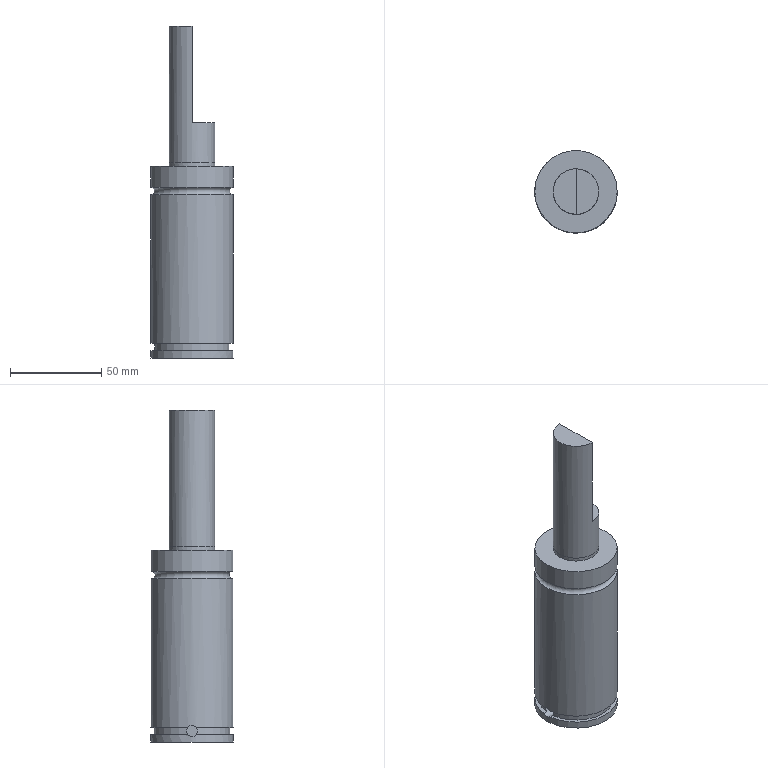Part | NX | features solid 2 | 1 solid | 16 faces | box 45.2 x 45.2 x 182 mm | volume 191111 mm3 | plane 8 | cylinder 7 | torus 1 | commonest cylinder face diameters 45.2 x3 6 x1 24.98 x1 25 x1 41.2 x1
STEP:
#1=CARTESIAN_POINT('',(-447.489,-357.236,-202.));
#2=VERTEX_POINT('',#1);
#3=CARTESIAN_POINT('',(-447.489,-352.764,-202.));
#4=VERTEX_POINT('',#3);
#5=CARTESIAN_POINT('',(-425.,-355.,-202.));
#6=DIRECTION('',(0.,0.,-1.));
#7=DIRECTION('',(1.,0.,0.));
#8=AXIS2_PLACEMENT_3D('',#5,#6,#7);
#9=CIRCLE('',#8,22.6);
#10=EDGE_CURVE('',#2,#4,#9,.F.);
#11=ORIENTED_EDGE('',*,*,#10,.T.);
#12=CARTESIAN_POINT('',(-447.489,-352.764,-202.));
#13=CARTESIAN_POINT('',(-447.545,-353.325,-201.372));
#14=CARTESIAN_POINT('',(-447.655,-355.003,-200.628));
#15=CARTESIAN_POINT('',(-447.545,-356.675,-201.372));
#16=CARTESIAN_POINT('',(-447.489,-357.236,-202.));
#17=B_SPLINE_CURVE_WITH_KNOTS('',3,(#12,#13,#14,#15,#16),.UNSPECIFIED.,.F.,.F.,(4,1,4),(0.006877,0.009391,0.01191),.UNSPECIFIED.);
#18=EDGE_CURVE('',#4,#2,#17,.T.);
#19=ORIENTED_EDGE('',*,*,#18,.T.);
#20=EDGE_LOOP('',(#11,#19));
#21=FACE_BOUND('',#20,.T.);
#22=CARTESIAN_POINT('',(-402.4,-355.,-120.5));
#23=VERTEX_POINT('',#22);
#24=CARTESIAN_POINT('',(-425.,-355.,-120.5));
#25=DIRECTION('',(0.,0.,-1.));
#26=DIRECTION('',(1.,0.,0.));
#27=AXIS2_PLACEMENT_3D('',#24,#25,#26);
#28=CIRCLE('',#27,22.6);
#29=EDGE_CURVE('',#23,#23,#28,.T.);
#30=ORIENTED_EDGE('',*,*,#29,.T.);
#31=EDGE_LOOP('',(#30));
#32=FACE_BOUND('',#31,.T.);
#33=CARTESIAN_POINT('',(-425.,-355.,-105.));
#34=DIRECTION('',(0.,0.,-1.));
#35=DIRECTION('',(1.,0.,0.));
#36=AXIS2_PLACEMENT_3D('',#33,#34,#35);
#37=CYLINDRICAL_SURFACE('',#36,22.6);
#38=ADVANCED_FACE('',(#21,#32),#37,.T.);
#39=CARTESIAN_POINT('',(-447.6,-355.,-105.));
#40=VERTEX_POINT('',#39);
#41=CARTESIAN_POINT('',(-425.,-355.,-105.));
#42=DIRECTION('',(0.,0.,1.));
#43=DIRECTION('',(-1.,0.,0.));
#44=AXIS2_PLACEMENT_3D('',#41,#42,#43);
#45=CIRCLE('',#44,22.6);
#46=EDGE_CURVE('',#40,#40,#45,.T.);
#47=ORIENTED_EDGE('',*,*,#46,.T.);
#48=EDGE_LOOP('',(#47));
#49=FACE_BOUND('',#48,.T.);
#50=CARTESIAN_POINT('',(-437.5,-355.,-105.));
#51=VERTEX_POINT('',#50);
#52=CARTESIAN_POINT('',(-425.,-355.,-105.));
#53=DIRECTION('',(0.,0.,1.));
#54=DIRECTION('',(-1.,0.,0.));
#55=AXIS2_PLACEMENT_3D('',#52,#53,#54);
#56=CIRCLE('',#55,12.5);
#57=EDGE_CURVE('',#51,#51,#56,.T.);
#58=ORIENTED_EDGE('',*,*,#57,.F.);
#59=EDGE_LOOP('',(#58));
#60=FACE_BOUND('',#59,.T.);
#61=CARTESIAN_POINT('',(-425.,-355.,-105.));
#62=DIRECTION('',(0.,0.,1.));
#63=DIRECTION('',(-1.,0.,0.));
#64=AXIS2_PLACEMENT_3D('',#61,#62,#63);
#65=PLANE('',#64);
#66=ADVANCED_FACE('',(#49,#60),#65,.T.);
#67=CARTESIAN_POINT('',(-402.4,-355.,-116.5));
#68=VERTEX_POINT('',#67);
#69=CARTESIAN_POINT('',(-425.,-355.,-116.5));
#70=DIRECTION('',(0.,0.,-1.));
#71=DIRECTION('',(1.,0.,0.));
#72=AXIS2_PLACEMENT_3D('',#69,#70,#71);
#73=CIRCLE('',#72,22.6);
#74=EDGE_CURVE('',#68,#68,#73,.F.);
#75=ORIENTED_EDGE('',*,*,#74,.T.);
#76=EDGE_LOOP('',(#75));
#77=FACE_BOUND('',#76,.T.);
#78=ORIENTED_EDGE('',*,*,#46,.F.);
#79=EDGE_LOOP('',(#78));
#80=FACE_BOUND('',#79,.T.);
#81=CARTESIAN_POINT('',(-425.,-355.,-105.));
#82=DIRECTION('',(0.,0.,-1.));
#83=DIRECTION('',(1.,0.,0.));
#84=AXIS2_PLACEMENT_3D('',#81,#82,#83);
#85=CYLINDRICAL_SURFACE('',#84,22.6);
#86=ADVANCED_FACE('',(#77,#80),#85,.T.);
#87=CARTESIAN_POINT('',(-433.818,-346.154,-103.));
#88=VERTEX_POINT('',#87);
#89=CARTESIAN_POINT('',(-438.852,-354.978,-103.));
#90=CARTESIAN_POINT('',(-434.78,-345.19,-103.));
#91=CARTESIAN_POINT('',(-424.978,-341.148,-103.));
#92=CARTESIAN_POINT('',(-415.19,-345.22,-103.));
#93=CARTESIAN_POINT('',(-411.148,-355.022,-103.));
#94=CARTESIAN_POINT('',(-415.22,-364.81,-103.));
#95=CARTESIAN_POINT('',(-425.022,-368.852,-103.));
#96=CARTESIAN_POINT('',(-434.81,-364.78,-103.));
#97=CARTESIAN_POINT('',(-438.852,-354.978,-103.));
#98=CARTESIAN_POINT('',(-434.78,-345.19,-103.));
#99=CARTESIAN_POINT('',(-424.978,-341.148,-103.));
#100=B_SPLINE_CURVE_WITH_KNOTS('',3,(#89,#90,#91,#92,#93,#94,#95,#96,#97,#98,#99),.UNSPECIFIED.,.T.,.F.,(1,1,1,1,1,1,1,1,1,1,1,1,1,1,1),(-0.2498,-0.1248,0.0002479,0.1252,0.2502,0.3752,0.5002,0.6252,0.7502,0.8752,1.,1.125,1.25,1.375,1.5),.UNSPECIFIED.);
#101=EDGE_CURVE('',#88,#88,#100,.F.);
#102=ORIENTED_EDGE('',*,*,#101,.F.);
#103=EDGE_LOOP('',(#102));
#104=FACE_BOUND('',#103,.T.);
#105=ORIENTED_EDGE('',*,*,#57,.T.);
#106=EDGE_LOOP('',(#105));
#107=FACE_BOUND('',#106,.T.);
#108=CARTESIAN_POINT('',(-425.,-355.,-103.));
#109=DIRECTION('',(0.,0.,-1.));
#110=DIRECTION('',(1.,0.,0.));
#111=AXIS2_PLACEMENT_3D('',#108,#109,#110);
#112=CYLINDRICAL_SURFACE('',#111,12.5);
#113=ADVANCED_FACE('',(#104,#107),#112,.T.);
#114=ORIENTED_EDGE('',*,*,#74,.F.);
#115=EDGE_LOOP('',(#114));
#116=FACE_BOUND('',#115,.T.);
#117=ORIENTED_EDGE('',*,*,#29,.F.);
#118=EDGE_LOOP('',(#117));
#119=FACE_BOUND('',#118,.T.);
#120=CARTESIAN_POINT('',(-425.,-355.,-118.5));
#121=DIRECTION('',(0.,0.,-1.));
#122=DIRECTION('',(1.,0.,0.));
#123=AXIS2_PLACEMENT_3D('',#120,#121,#122);
#124=TOROIDAL_SURFACE('',#123,22.6,2.);
#125=ADVANCED_FACE('',(#116,#119),#124,.F.);
#126=ORIENTED_EDGE('',*,*,#10,.F.);
#127=CARTESIAN_POINT('',(-445.478,-357.236,-202.));
#128=VERTEX_POINT('',#127);
#129=CARTESIAN_POINT('',(-440.1,-357.236,-202.));
#130=DIRECTION('',(-1.,0.,0.));
#131=VECTOR('',#130,1000.);
#132=LINE('',#129,#131);
#133=EDGE_CURVE('',#2,#128,#132,.F.);
#134=ORIENTED_EDGE('',*,*,#133,.T.);
#135=CARTESIAN_POINT('',(-445.478,-352.764,-202.));
#136=VERTEX_POINT('',#135);
#137=CARTESIAN_POINT('',(-425.,-355.,-202.));
#138=DIRECTION('',(0.,0.,1.));
#139=DIRECTION('',(-1.,0.,0.));
#140=AXIS2_PLACEMENT_3D('',#137,#138,#139);
#141=CIRCLE('',#140,20.6);
#142=EDGE_CURVE('',#128,#136,#141,.T.);
#143=ORIENTED_EDGE('',*,*,#142,.T.);
#144=CARTESIAN_POINT('',(-440.1,-352.764,-202.));
#145=DIRECTION('',(-1.,0.,0.));
#146=VECTOR('',#145,1000.);
#147=LINE('',#144,#146);
#148=EDGE_CURVE('',#136,#4,#147,.T.);
#149=ORIENTED_EDGE('',*,*,#148,.T.);
#150=EDGE_LOOP('',(#126,#134,#143,#149));
#151=FACE_BOUND('',#150,.T.);
#152=CARTESIAN_POINT('',(-425.,-355.,-202.));
#153=DIRECTION('',(0.,0.,-1.));
#154=DIRECTION('',(1.,0.,0.));
#155=AXIS2_PLACEMENT_3D('',#152,#153,#154);
#156=PLANE('',#155);
#157=ADVANCED_FACE('',(#151),#156,.T.);
#158=CARTESIAN_POINT('',(-445.478,-357.236,-206.));
#159=VERTEX_POINT('',#158);
#160=CARTESIAN_POINT('',(-445.478,-352.764,-206.));
#161=VERTEX_POINT('',#160);
#162=CARTESIAN_POINT('',(-425.,-355.,-206.));
#163=DIRECTION('',(0.,0.,1.));
#164=DIRECTION('',(-1.,0.,0.));
#165=AXIS2_PLACEMENT_3D('',#162,#163,#164);
#166=CIRCLE('',#165,20.6);
#167=EDGE_CURVE('',#159,#161,#166,.T.);
#168=ORIENTED_EDGE('',*,*,#167,.F.);
#169=CARTESIAN_POINT('',(-447.489,-357.236,-206.));
#170=VERTEX_POINT('',#169);
#171=CARTESIAN_POINT('',(-440.1,-357.236,-206.));
#172=DIRECTION('',(-1.,0.,0.));
#173=VECTOR('',#172,1000.);
#174=LINE('',#171,#173);
#175=EDGE_CURVE('',#159,#170,#174,.T.);
#176=ORIENTED_EDGE('',*,*,#175,.T.);
#177=CARTESIAN_POINT('',(-447.489,-352.764,-206.));
#178=VERTEX_POINT('',#177);
#179=CARTESIAN_POINT('',(-425.,-355.,-206.));
#180=DIRECTION('',(0.,0.,-1.));
#181=DIRECTION('',(1.,0.,0.));
#182=AXIS2_PLACEMENT_3D('',#179,#180,#181);
#183=CIRCLE('',#182,22.6);
#184=EDGE_CURVE('',#178,#170,#183,.T.);
#185=ORIENTED_EDGE('',*,*,#184,.F.);
#186=CARTESIAN_POINT('',(-440.1,-352.764,-206.));
#187=DIRECTION('',(-1.,0.,0.));
#188=VECTOR('',#187,1000.);
#189=LINE('',#186,#188);
#190=EDGE_CURVE('',#178,#161,#189,.F.);
#191=ORIENTED_EDGE('',*,*,#190,.T.);
#192=EDGE_LOOP('',(#168,#176,#185,#191));
#193=FACE_BOUND('',#192,.T.);
#194=CARTESIAN_POINT('',(-425.,-355.,-206.));
#195=DIRECTION('',(0.,0.,-1.));
#196=DIRECTION('',(1.,0.,0.));
#197=AXIS2_PLACEMENT_3D('',#194,#195,#196);
#198=PLANE('',#197);
#199=ADVANCED_FACE('',(#193),#198,.F.);
#200=CARTESIAN_POINT('',(-445.478,-357.236,-206.));
#201=CARTESIAN_POINT('',(-445.425,-357.72,-205.459));
#202=CARTESIAN_POINT('',(-445.335,-358.279,-203.999));
#203=CARTESIAN_POINT('',(-445.425,-357.723,-202.545));
#204=CARTESIAN_POINT('',(-445.478,-357.236,-202.));
#205=B_SPLINE_CURVE_WITH_KNOTS('',3,(#200,#201,#202,#203,#204),.UNSPECIFIED.,.F.,.F.,(4,1,4),(0.002515,0.004697,0.006878),.UNSPECIFIED.);
#206=EDGE_CURVE('',#159,#128,#205,.T.);
#207=ORIENTED_EDGE('',*,*,#206,.F.);
#208=ORIENTED_EDGE('',*,*,#167,.T.);
#209=CARTESIAN_POINT('',(-445.478,-352.764,-202.));
#210=CARTESIAN_POINT('',(-445.425,-352.277,-202.544));
#211=CARTESIAN_POINT('',(-445.336,-351.722,-203.999));
#212=CARTESIAN_POINT('',(-445.425,-352.278,-205.457));
#213=CARTESIAN_POINT('',(-445.478,-352.764,-206.));
#214=B_SPLINE_CURVE_WITH_KNOTS('',3,(#209,#210,#211,#212,#213),.UNSPECIFIED.,.F.,.F.,(4,1,4),(0.01191,0.01409,0.01627),.UNSPECIFIED.);
#215=EDGE_CURVE('',#136,#161,#214,.T.);
#216=ORIENTED_EDGE('',*,*,#215,.F.);
#217=ORIENTED_EDGE('',*,*,#142,.F.);
#218=EDGE_LOOP('',(#207,#208,#216,#217));
#219=FACE_BOUND('',#218,.T.);
#220=CARTESIAN_POINT('',(-425.,-355.,-206.));
#221=DIRECTION('',(0.,0.,1.));
#222=DIRECTION('',(-1.,0.,0.));
#223=AXIS2_PLACEMENT_3D('',#220,#221,#222);
#224=CYLINDRICAL_SURFACE('',#223,20.6);
#225=ADVANCED_FACE('',(#219),#224,.T.);
#226=CARTESIAN_POINT('',(-447.6,-355.,-210.));
#227=VERTEX_POINT('',#226);
#228=CARTESIAN_POINT('',(-425.,-355.,-210.));
#229=DIRECTION('',(0.,0.,1.));
#230=DIRECTION('',(-1.,0.,0.));
#231=AXIS2_PLACEMENT_3D('',#228,#229,#230);
#232=CIRCLE('',#231,22.6);
#233=EDGE_CURVE('',#227,#227,#232,.T.);
#234=ORIENTED_EDGE('',*,*,#233,.F.);
#235=EDGE_LOOP('',(#234));
#236=FACE_BOUND('',#235,.T.);
#237=CARTESIAN_POINT('',(-425.,-355.,-210.));
#238=DIRECTION('',(0.,0.,1.));
#239=DIRECTION('',(-1.,0.,0.));
#240=AXIS2_PLACEMENT_3D('',#237,#238,#239);
#241=PLANE('',#240);
#242=ADVANCED_FACE('',(#236),#241,.F.);
#243=ORIENTED_EDGE('',*,*,#184,.T.);
#244=CARTESIAN_POINT('',(-447.489,-357.236,-206.));
#245=CARTESIAN_POINT('',(-447.545,-356.671,-206.631));
#246=CARTESIAN_POINT('',(-447.655,-355.,-207.369));
#247=CARTESIAN_POINT('',(-447.545,-353.329,-206.631));
#248=CARTESIAN_POINT('',(-447.489,-352.764,-206.));
#249=B_SPLINE_CURVE_WITH_KNOTS('',3,(#244,#245,#246,#247,#248),.UNSPECIFIED.,.F.,.F.,(4,1,4),(-0.002511,-0.000000091,0.00251),.UNSPECIFIED.);
#250=EDGE_CURVE('',#170,#178,#249,.T.);
#251=ORIENTED_EDGE('',*,*,#250,.T.);
#252=EDGE_LOOP('',(#243,#251));
#253=FACE_BOUND('',#252,.T.);
#254=ORIENTED_EDGE('',*,*,#233,.T.);
#255=EDGE_LOOP('',(#254));
#256=FACE_BOUND('',#255,.T.);
#257=CARTESIAN_POINT('',(-425.,-355.,-105.));
#258=DIRECTION('',(0.,0.,-1.));
#259=DIRECTION('',(1.,0.,0.));
#260=AXIS2_PLACEMENT_3D('',#257,#258,#259);
#261=CYLINDRICAL_SURFACE('',#260,22.6);
#262=ADVANCED_FACE('',(#253,#256),#261,.T.);
#263=CARTESIAN_POINT('',(-440.1,-358.,-204.));
#264=VERTEX_POINT('',#263);
#265=CARTESIAN_POINT('',(-440.1,-355.,-204.));
#266=DIRECTION('',(-1.,0.,0.));
#267=DIRECTION('',(0.,-1.,0.));
#268=AXIS2_PLACEMENT_3D('',#265,#266,#267);
#269=CIRCLE('',#268,3.);
#270=EDGE_CURVE('',#264,#264,#269,.T.);
#271=ORIENTED_EDGE('',*,*,#270,.F.);
#272=EDGE_LOOP('',(#271));
#273=FACE_BOUND('',#272,.T.);
#274=ORIENTED_EDGE('',*,*,#148,.F.);
#275=ORIENTED_EDGE('',*,*,#215,.T.);
#276=ORIENTED_EDGE('',*,*,#190,.F.);
#277=ORIENTED_EDGE('',*,*,#250,.F.);
#278=ORIENTED_EDGE('',*,*,#175,.F.);
#279=ORIENTED_EDGE('',*,*,#206,.T.);
#280=ORIENTED_EDGE('',*,*,#133,.F.);
#281=ORIENTED_EDGE('',*,*,#18,.F.);
#282=EDGE_LOOP('',(#274,#275,#276,#277,#278,#279,#280,#281));
#283=FACE_BOUND('',#282,.T.);
#284=CARTESIAN_POINT('',(-440.1,-355.,-204.));
#285=DIRECTION('',(-1.,0.,0.));
#286=DIRECTION('',(0.,0.,-1.));
#287=AXIS2_PLACEMENT_3D('',#284,#285,#286);
#288=CYLINDRICAL_SURFACE('',#287,3.);
#289=ADVANCED_FACE('',(#273,#283),#288,.F.);
#290=ORIENTED_EDGE('',*,*,#270,.T.);
#291=EDGE_LOOP('',(#290));
#292=FACE_BOUND('',#291,.T.);
#293=CARTESIAN_POINT('',(-440.1,-355.,-204.));
#294=DIRECTION('',(-1.,0.,0.));
#295=DIRECTION('',(0.,0.,-1.));
#296=AXIS2_PLACEMENT_3D('',#293,#294,#295);
#297=PLANE('',#296);
#298=ADVANCED_FACE('',(#292),#297,.T.);
#299=ORIENTED_EDGE('',*,*,#101,.T.);
#300=EDGE_LOOP('',(#299));
#301=FACE_BOUND('',#300,.T.);
#302=CARTESIAN_POINT('',(-425.,-367.5,-28.));
#303=VERTEX_POINT('',#302);
#304=CARTESIAN_POINT('',(-425.,-367.5,-81.));
#305=VERTEX_POINT('',#304);
#306=CARTESIAN_POINT('',(-425.,-367.49,-28.));
#307=DIRECTION('',(0.,0.,-1.));
#308=VECTOR('',#307,1000.);
#309=LINE('',#306,#308);
#310=EDGE_CURVE('',#303,#305,#309,.T.);
#311=ORIENTED_EDGE('',*,*,#310,.F.);
#312=CARTESIAN_POINT('',(-425.,-342.5,-28.));
#313=VERTEX_POINT('',#312);
#314=CARTESIAN_POINT('',(-425.,-355.,-28.));
#315=DIRECTION('',(0.,0.,1.));
#316=DIRECTION('',(-1.,0.,0.));
#317=AXIS2_PLACEMENT_3D('',#314,#315,#316);
#318=CIRCLE('',#317,12.49);
#319=EDGE_CURVE('',#313,#303,#318,.T.);
#320=ORIENTED_EDGE('',*,*,#319,.F.);
#321=CARTESIAN_POINT('',(-425.,-342.5,-81.));
#322=VERTEX_POINT('',#321);
#323=CARTESIAN_POINT('',(-425.,-342.51,-81.));
#324=DIRECTION('',(0.,0.,-1.));
#325=VECTOR('',#324,1000.);
#326=LINE('',#323,#325);
#327=EDGE_CURVE('',#322,#313,#326,.F.);
#328=ORIENTED_EDGE('',*,*,#327,.F.);
#329=CARTESIAN_POINT('',(-425.,-355.,-81.));
#330=DIRECTION('',(0.,0.,-1.));
#331=DIRECTION('',(1.,0.,0.));
#332=AXIS2_PLACEMENT_3D('',#329,#330,#331);
#333=CIRCLE('',#332,12.49);
#334=EDGE_CURVE('',#322,#305,#333,.T.);
#335=ORIENTED_EDGE('',*,*,#334,.T.);
#336=EDGE_LOOP('',(#311,#320,#328,#335));
#337=FACE_BOUND('',#336,.T.);
#338=CARTESIAN_POINT('',(-425.,-355.,-28.));
#339=DIRECTION('',(0.,0.,-1.));
#340=DIRECTION('',(1.,0.,0.));
#341=AXIS2_PLACEMENT_3D('',#338,#339,#340);
#342=CYLINDRICAL_SURFACE('',#341,12.49);
#343=ADVANCED_FACE('',(#301,#337),#342,.T.);
#344=ORIENTED_EDGE('',*,*,#319,.T.);
#345=CARTESIAN_POINT('',(-425.,-537.203,-28.));
#346=DIRECTION('',(0.,1.,0.));
#347=VECTOR('',#346,1000.);
#348=LINE('',#345,#347);
#349=EDGE_CURVE('',#303,#313,#348,.T.);
#350=ORIENTED_EDGE('',*,*,#349,.T.);
#351=EDGE_LOOP('',(#344,#350));
#352=FACE_BOUND('',#351,.T.);
#353=CARTESIAN_POINT('',(-425.,-355.,-28.));
#354=DIRECTION('',(0.,0.,1.));
#355=DIRECTION('',(-1.,0.,0.));
#356=AXIS2_PLACEMENT_3D('',#353,#354,#355);
#357=PLANE('',#356);
#358=ADVANCED_FACE('',(#352),#357,.T.);
#359=CARTESIAN_POINT('',(-425.,-537.203,-81.));
#360=DIRECTION('',(0.,1.,0.));
#361=VECTOR('',#360,1000.);
#362=LINE('',#359,#361);
#363=EDGE_CURVE('',#305,#322,#362,.T.);
#364=ORIENTED_EDGE('',*,*,#363,.F.);
#365=ORIENTED_EDGE('',*,*,#334,.F.);
#366=EDGE_LOOP('',(#364,#365));
#367=FACE_BOUND('',#366,.T.);
#368=CARTESIAN_POINT('',(-425.,-537.203,-81.));
#369=DIRECTION('',(0.,0.,-1.));
#370=DIRECTION('',(1.,0.,0.));
#371=AXIS2_PLACEMENT_3D('',#368,#369,#370);
#372=PLANE('',#371);
#373=ADVANCED_FACE('',(#367),#372,.F.);
#374=ORIENTED_EDGE('',*,*,#310,.T.);
#375=ORIENTED_EDGE('',*,*,#363,.T.);
#376=ORIENTED_EDGE('',*,*,#327,.T.);
#377=ORIENTED_EDGE('',*,*,#349,.F.);
#378=EDGE_LOOP('',(#374,#375,#376,#377));
#379=FACE_BOUND('',#378,.T.);
#380=CARTESIAN_POINT('',(-425.,-537.203,-81.));
#381=DIRECTION('',(1.,0.,0.));
#382=DIRECTION('',(0.,1.,0.));
#383=AXIS2_PLACEMENT_3D('',#380,#381,#382);
#384=PLANE('',#383);
#385=ADVANCED_FACE('',(#379),#384,.T.);
#386=CLOSED_SHELL('',(#38,#66,#86,#113,#125,#157,#199,#225,#242,#262,#289,#298,#343,#358,#373,#385));
#387=MANIFOLD_SOLID_BREP('',#386);
#388=(LENGTH_UNIT()NAMED_UNIT(*)SI_UNIT(.MILLI.,.METRE.));
#389=UNCERTAINTY_MEASURE_WITH_UNIT(LENGTH_MEASURE(0.0508),#388,'','');
#390=(NAMED_UNIT(*)PLANE_ANGLE_UNIT()SI_UNIT($,.RADIAN.));
#391=(NAMED_UNIT(*)SI_UNIT($,.STERADIAN.)SOLID_ANGLE_UNIT());
#392=(GEOMETRIC_REPRESENTATION_CONTEXT(3)GLOBAL_UNCERTAINTY_ASSIGNED_CONTEXT((#389))GLOBAL_UNIT_ASSIGNED_CONTEXT((#388,#390,#391))REPRESENTATION_CONTEXT('',''));
#393=ADVANCED_BREP_SHAPE_REPRESENTATION('',(#387),#392);